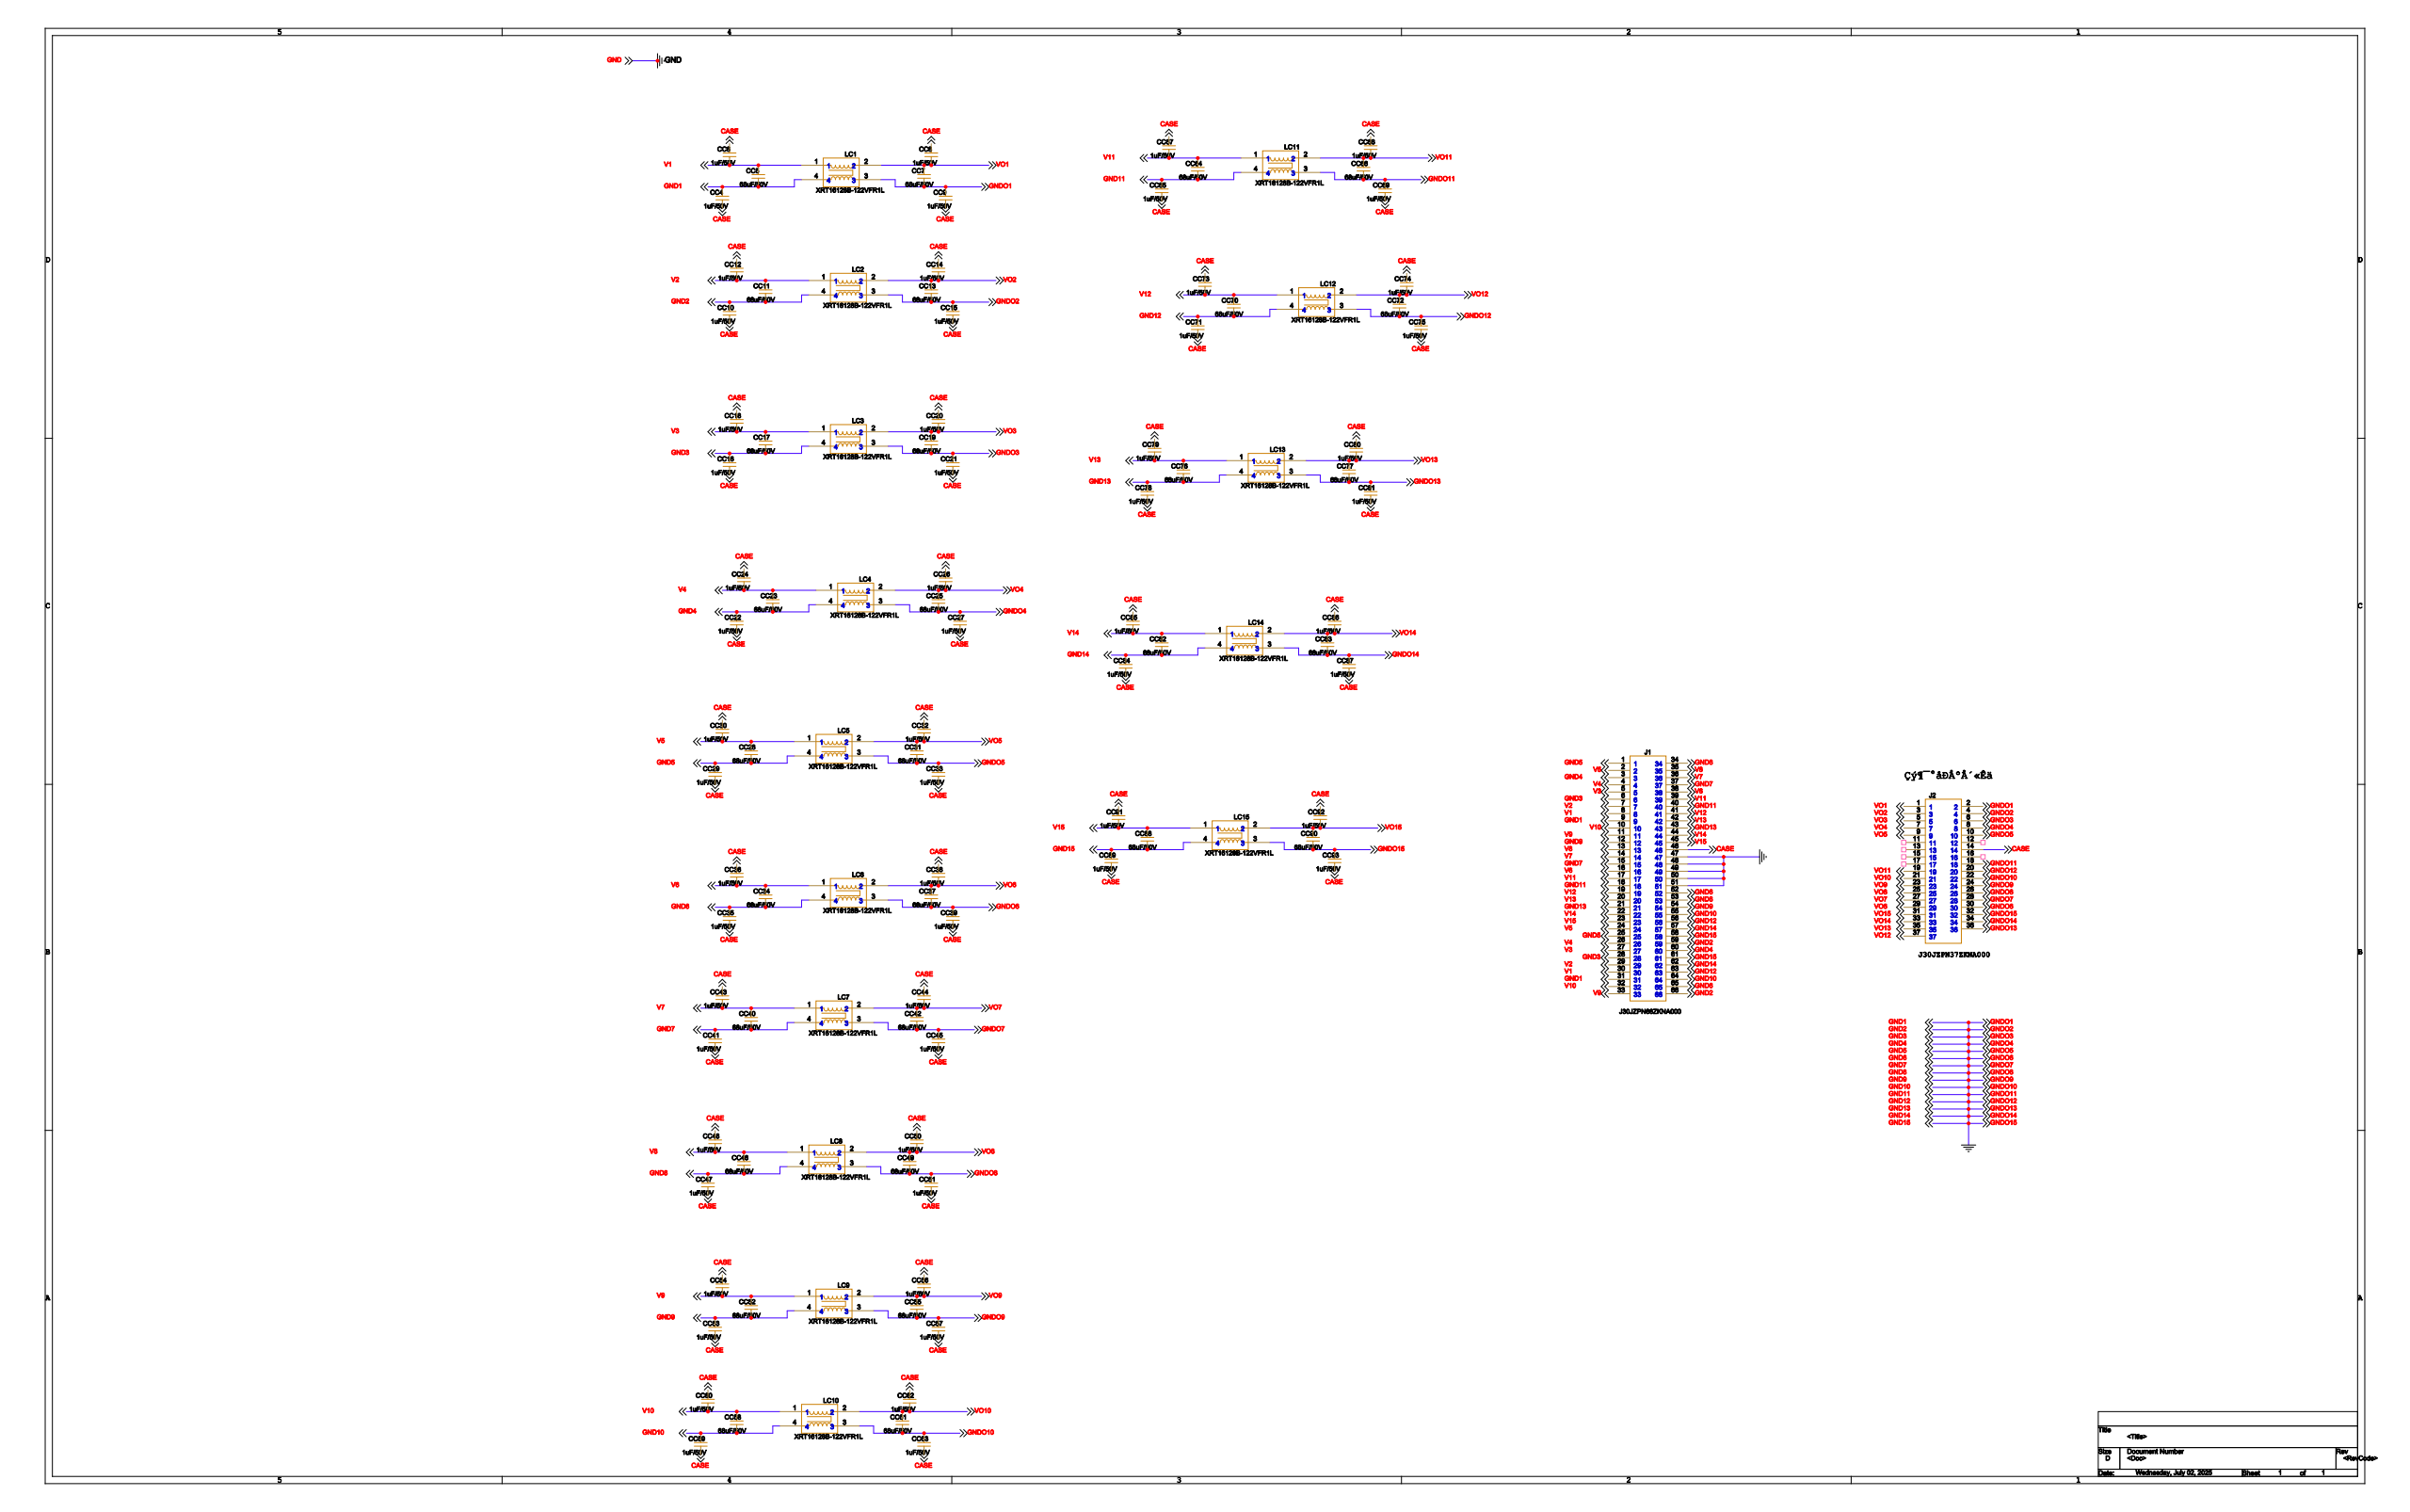Circuit board | Cadence Allegro | 107 parts | 32 nets
Bill of materials:
SYM_NAME,COMP_DEVICE_TYPE,COMP_VALUE,COMP_TOL,COMP_CLASS,REFDES
C0603,CAP NP_C0603_1UF/50V,1uF/50V,,IC,CC4
C1812,CAP NP_C1812_68UF/50V,68uF/50V,,IC,CC5
C0603,CAP NP_C0603_1UF/50V,1uF/50V,,IC,CC6
C1812,CAP NP_C1812_68UF/50V,68uF/50V,,IC,CC7
C0603,CAP NP_C0603_1UF/50V,1uF/50V,,IC,CC8
C0603,CAP NP_C0603_1UF/50V,1uF/50V,,IC,CC9
C0603,CAP NP_C0603_1UF/50V,1uF/50V,,IC,CC10
C1812,CAP NP_C1812_68UF/50V,68uF/50V,,IC,CC11
C0603,CAP NP_C0603_1UF/50V,1uF/50V,,IC,CC12
C1812,CAP NP_C1812_68UF/50V,68uF/50V,,IC,CC13
C0603,CAP NP_C0603_1UF/50V,1uF/50V,,IC,CC14
C0603,CAP NP_C0603_1UF/50V,1uF/50V,,IC,CC15
C0603,CAP NP_C0603_1UF/50V,1uF/50V,,IC,CC16
C1812,CAP NP_C1812_68UF/50V,68uF/50V,,IC,CC17
C0603,CAP NP_C0603_1UF/50V,1uF/50V,,IC,CC18
C1812,CAP NP_C1812_68UF/50V,68uF/50V,,IC,CC19
C0603,CAP NP_C0603_1UF/50V,1uF/50V,,IC,CC20
C0603,CAP NP_C0603_1UF/50V,1uF/50V,,IC,CC21
C0603,CAP NP_C0603_1UF/50V,1uF/50V,,IC,CC22
C1812,CAP NP_C1812_68UF/50V,68uF/50V,,IC,CC23
C0603,CAP NP_C0603_1UF/50V,1uF/50V,,IC,CC24
C1812,CAP NP_C1812_68UF/50V,68uF/50V,,IC,CC25
C0603,CAP NP_C0603_1UF/50V,1uF/50V,,IC,CC26
C0603,CAP NP_C0603_1UF/50V,1uF/50V,,IC,CC27
C1812,CAP NP_C1812_68UF/50V,68uF/50V,,IC,CC28
C0603,CAP NP_C0603_1UF/50V,1uF/50V,,IC,CC29
C0603,CAP NP_C0603_1UF/50V,1uF/50V,,IC,CC30
C1812,CAP NP_C1812_68UF/50V,68uF/50V,,IC,CC31
C0603,CAP NP_C0603_1UF/50V,1uF/50V,,IC,CC32
C0603,CAP NP_C0603_1UF/50V,1uF/50V,,IC,CC33
C1812,CAP NP_C1812_68UF/50V,68uF/50V,,IC,CC34
C0603,CAP NP_C0603_1UF/50V,1uF/50V,,IC,CC35
C0603,CAP NP_C0603_1UF/50V,1uF/50V,,IC,CC36
C1812,CAP NP_C1812_68UF/50V,68uF/50V,,IC,CC37
C0603,CAP NP_C0603_1UF/50V,1uF/50V,,IC,CC38
C0603,CAP NP_C0603_1UF/50V,1uF/50V,,IC,CC39
C1812,CAP NP_C1812_68UF/50V,68uF/50V,,IC,CC40
C0603,CAP NP_C0603_1UF/50V,1uF/50V,,IC,CC41
C1812,CAP NP_C1812_68UF/50V,68uF/50V,,IC,CC42
C0603,CAP NP_C0603_1UF/50V,1uF/50V,,IC,CC43
C0603,CAP NP_C0603_1UF/50V,1uF/50V,,IC,CC44
C0603,CAP NP_C0603_1UF/50V,1uF/50V,,IC,CC45
C1812,CAP NP_C1812_68UF/50V,68uF/50V,,IC,CC46
C0603,CAP NP_C0603_1UF/50V,1uF/50V,,IC,CC47
C0603,CAP NP_C0603_1UF/50V,1uF/50V,,IC,CC48
C1812,CAP NP_C1812_68UF/50V,68uF/50V,,IC,CC49
C0603,CAP NP_C0603_1UF/50V,1uF/50V,,IC,CC50
C0603,CAP NP_C0603_1UF/50V,1uF/50V,,IC,CC51
C1812,CAP NP_C1812_68UF/50V,68uF/50V,,IC,CC52
C0603,CAP NP_C0603_1UF/50V,1uF/50V,,IC,CC53
C0603,CAP NP_C0603_1UF/50V,1uF/50V,,IC,CC54
C1812,CAP NP_C1812_68UF/50V,68uF/50V,,IC,CC55
C0603,CAP NP_C0603_1UF/50V,1uF/50V,,IC,CC56
C0603,CAP NP_C0603_1UF/50V,1uF/50V,,IC,CC57
C1812,CAP NP_C1812_68UF/50V,68uF/50V,,IC,CC58
C0603,CAP NP_C0603_1UF/50V,1uF/50V,,IC,CC59
C0603,CAP NP_C0603_1UF/50V,1uF/50V,,IC,CC60
C1812,CAP NP_C1812_68UF/50V,68uF/50V,,IC,CC61
C0603,CAP NP_C0603_1UF/50V,1uF/50V,,IC,CC62
C0603,CAP NP_C0603_1UF/50V,1uF/50V,,IC,CC63
C1812,CAP NP_C1812_68UF/50V,68uF/50V,,IC,CC64
C0603,CAP NP_C0603_1UF/50V,1uF/50V,,IC,CC65
C1812,CAP NP_C1812_68UF/50V,68uF/50V,,IC,CC66
C0603,CAP NP_C0603_1UF/50V,1uF/50V,,IC,CC67
C0603,CAP NP_C0603_1UF/50V,1uF/50V,,IC,CC68
C0603,CAP NP_C0603_1UF/50V,1uF/50V,,IC,CC69
C1812,CAP NP_C1812_68UF/50V,68uF/50V,,IC,CC70
C0603,CAP NP_C0603_1UF/50V,1uF/50V,,IC,CC71
C1812,CAP NP_C1812_68UF/50V,68uF/50V,,IC,CC72
C0603,CAP NP_C0603_1UF/50V,1uF/50V,,IC,CC73
C0603,CAP NP_C0603_1UF/50V,1uF/50V,,IC,CC74
C0603,CAP NP_C0603_1UF/50V,1uF/50V,,IC,CC75
C1812,CAP NP_C1812_68UF/50V,68uF/50V,,IC,CC76
C1812,CAP NP_C1812_68UF/50V,68uF/50V,,IC,CC77
C0603,CAP NP_C0603_1UF/50V,1uF/50V,,IC,CC78
C0603,CAP NP_C0603_1UF/50V,1uF/50V,,IC,CC79
C0603,CAP NP_C0603_1UF/50V,1uF/50V,,IC,CC80
C0603,CAP NP_C0603_1UF/50V,1uF/50V,,IC,CC81
C1812,CAP NP_C1812_68UF/50V,68uF/50V,,IC,CC82
C1812,CAP NP_C1812_68UF/50V,68uF/50V,,IC,CC83
C0603,CAP NP_C0603_1UF/50V,1uF/50V,,IC,CC84
C0603,CAP NP_C0603_1UF/50V,1uF/50V,,IC,CC85
C0603,CAP NP_C0603_1UF/50V,1uF/50V,,IC,CC86
C0603,CAP NP_C0603_1UF/50V,1uF/50V,,IC,CC87
C1812,CAP NP_C1812_68UF/50V,68uF/50V,,IC,CC88
C0603,CAP NP_C0603_1UF/50V,1uF/50V,,IC,CC89
C1812,CAP NP_C1812_68UF/50V,68uF/50V,,IC,CC90
C0603,CAP NP_C0603_1UF/50V,1uF/50V,,IC,CC91
C0603,CAP NP_C0603_1UF/50V,1uF/50V,,IC,CC92
C0603,CAP NP_C0603_1UF/50V,1uF/50V,,IC,CC93
J30JZ66,J30JZ66_J30JZ66_J30JZPN66ZKNA00,J30JZPN66ZKNA000,,IC,J1
J30JZLN37,HJ30J-30ZKWP_0_J30JZLN37_J63A,J63A,,IC,J2
XRT16128B-122VFR1L,ACT45B_110_0_XRT16128B-122VFR1L,XRT16128B-122VFR1L,,IC,LC1
XRT16128B-122VFR1L,ACT45B_110_0_XRT16128B-122VFR1L,XRT16128B-122VFR1L,,IC,LC2
XRT16128B-122VFR1L,ACT45B_110_0_XRT16128B-122VFR1L,XRT16128B-122VFR1L,,IC,LC3
XRT16128B-122VFR1L,ACT45B_110_0_XRT16128B-122VFR1L,XRT16128B-122VFR1L,,IC,LC4
XRT16128B-122VFR1L,ACT45B_110_0_XRT16128B-122VFR1L,XRT16128B-122VFR1L,,IC,LC5
XRT16128B-122VFR1L,ACT45B_110_0_XRT16128B-122VFR1L,XRT16128B-122VFR1L,,IC,LC6
XRT16128B-122VFR1L,ACT45B_110_0_XRT16128B-122VFR1L,XRT16128B-122VFR1L,,IC,LC7
XRT16128B-122VFR1L,ACT45B_110_0_XRT16128B-122VFR1L,XRT16128B-122VFR1L,,IC,LC8
XRT16128B-122VFR1L,ACT45B_110_0_XRT16128B-122VFR1L,XRT16128B-122VFR1L,,IC,LC9
XRT16128B-122VFR1L,ACT45B_110_0_XRT16128B-122VFR1L,XRT16128B-122VFR1L,,IC,LC10
XRT16128B-122VFR1L,ACT45B_110_0_XRT16128B-122VFR1L,XRT16128B-122VFR1L,,IC,LC11
XRT16128B-122VFR1L,ACT45B_110_0_XRT16128B-122VFR1L,XRT16128B-122VFR1L,,IC,LC12
XRT16128B-122VFR1L,ACT45B_110_0_XRT16128B-122VFR1L,XRT16128B-122VFR1L,,IC,LC13
XRT16128B-122VFR1L,ACT45B_110_0_XRT16128B-122VFR1L,XRT16128B-122VFR1L,,IC,LC14
XRT16128B-122VFR1L,ACT45B_110_0_XRT16128B-122VFR1L,XRT16128B-122VFR1L,,IC,LC15
Netlist (net: part-pin ...):
V1: CC5-2 CC6-1 J1-8 J1-30 LC1-1
VO1: CC7-2 CC8-1 J2-1 LC1-2
GND: CC4-2 CC5-1 CC7-1 CC9-2 CC10-2 CC11-1 CC13-1 CC15-2 CC16-2 CC17-1 CC19-1 CC21-2 CC22-2 CC23-1 CC25-1 CC27-2 CC28-1 CC29-2 CC31-1 CC33-2 CC34-1 CC35-2 CC37-1 CC39-2 CC40-1 CC41-2 CC42-1 CC45-2 CC46-1 CC47-2 CC49-1 CC51-2 CC52-1 CC53-2 CC55-1 CC57-2 CC58-1 CC59-2 CC61-1 CC63-2 CC64-1 CC65-2 CC66-1 CC69-2 CC70-1 CC71-2 CC72-1 CC75-2 CC76-1 CC77-1 CC78-2 CC81-2 CC82-1 CC83-1 CC84-2 CC87-2 CC88-1 CC89-2 CC90-1 CC93-2 J1-1 J1-3 J1-6 J1-9 J1-12 J1-15 J1-18 J1-21 J1-25 J1-28 J1-31 J1-34 J1-37 J1-40 J1-43 J1-47 J1-48 J1-49 J1-50 J1-51 J1-52 J1-53 J1-54 J1-55 J1-56 J1-57 J1-58 J1-59 J1-60 J1-61 J1-62 J1-63 J1-64 J1-65 J1-66 J2-2 J2-4 J2-6 J2-8 J2-10 J2-18 J2-20 J2-22 J2-24 J2-26 J2-28 J2-30 J2-32 J2-34 J2-36 LC1-3 LC1-4 LC2-3 LC2-4 LC3-3 LC3-4 LC4-3 LC4-4 LC5-3 LC5-4 LC6-3 LC6-4 LC7-3 LC7-4 LC8-3 LC8-4 LC9-3 LC9-4 LC10-3 LC10-4 LC11-3 LC11-4 LC12-3 LC12-4 LC13-3 LC13-4 LC14-3 LC14-4 LC15-3 LC15-4
V10: CC58-2 CC60-1 J1-10 J1-32 LC10-1
VO10: CC61-2 CC62-1 J2-21 LC10-2
V11: CC64-2 CC67-1 J1-17 J1-39 LC11-1
VO11: CC66-2 CC68-1 J2-19 LC11-2
V12: CC70-2 CC73-1 J1-19 J1-41 LC12-1
VO12: CC72-2 CC74-1 J2-37 LC12-2
V13: CC76-2 CC79-1 J1-20 J1-42 LC13-1
VO13: CC77-2 CC80-1 J2-35 LC13-2
V14: CC82-2 CC85-1 J1-22 J1-44 LC14-1
VO14: CC83-2 CC86-1 J2-33 LC14-2
V15: CC88-2 CC91-1 J1-23 J1-45 LC15-1
VO15: CC90-2 CC92-1 J2-31 LC15-2
V2: CC11-2 CC12-1 J1-7 J1-29 LC2-1
VO2: CC13-2 CC14-1 J2-3 LC2-2
V3: CC17-2 CC18-1 J1-5 J1-27 LC3-1
VO3: CC19-2 CC20-1 J2-5 LC3-2
V4: CC23-2 CC24-1 J1-4 J1-26 LC4-1
VO4: CC25-2 CC26-1 J2-7 LC4-2
V5: CC28-2 CC30-1 J1-2 J1-24 LC5-1
VO5: CC31-2 CC32-1 J2-9 LC5-2
V6: CC34-2 CC36-1 J1-16 J1-38 LC6-1
VO6: CC37-2 CC38-1 J2-29 LC6-2
V7: CC40-2 CC43-1 J1-14 J1-36 LC7-1
VO7: CC42-2 CC44-1 J2-27 LC7-2
V8: CC46-2 CC48-1 J1-13 J1-35 LC8-1
VO8: CC49-2 CC50-1 J2-25 LC8-2
V9: CC52-2 CC54-1 J1-11 J1-33 LC9-1
VO9: CC55-2 CC56-1 J2-23 LC9-2
CASE: CC4-1 CC6-2 CC8-2 CC9-1 CC10-1 CC12-2 CC14-2 CC15-1 CC16-1 CC18-2 CC20-2 CC21-1 CC22-1 CC24-2 CC26-2 CC27-1 CC29-1 CC30-2 CC32-2 CC33-1 CC35-1 CC36-2 CC38-2 CC39-1 CC41-1 CC43-2 CC44-2 CC45-1 CC47-1 CC48-2 CC50-2 CC51-1 CC53-1 CC54-2 CC56-2 CC57-1 CC59-1 CC60-2 CC62-2 CC63-1 CC65-1 CC67-2 CC68-2 CC69-1 CC71-1 CC73-2 CC74-2 CC75-1 CC78-1 CC79-2 CC80-2 CC81-1 CC84-1 CC85-2 CC86-2 CC87-1 CC89-1 CC91-2 CC92-2 CC93-1 J1-46 J2-14